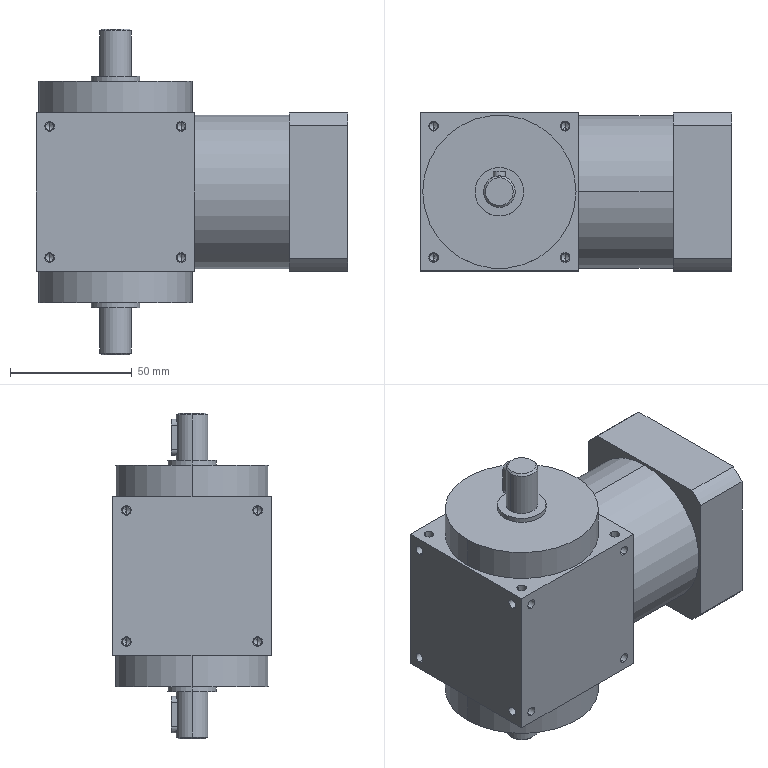Part | SolidWorks | features BaseBody 1 | 1 solid | 1800 faces | box 128 x 65 x 134 mm | volume 554755 mm3 | plane 1000 | spline 577 | cylinder 168 | cone 54 | torus 1 | commonest cylinder face diameters 4 x80 3.3 x40 5 x14 4.2 x8 63 x6 13 x4